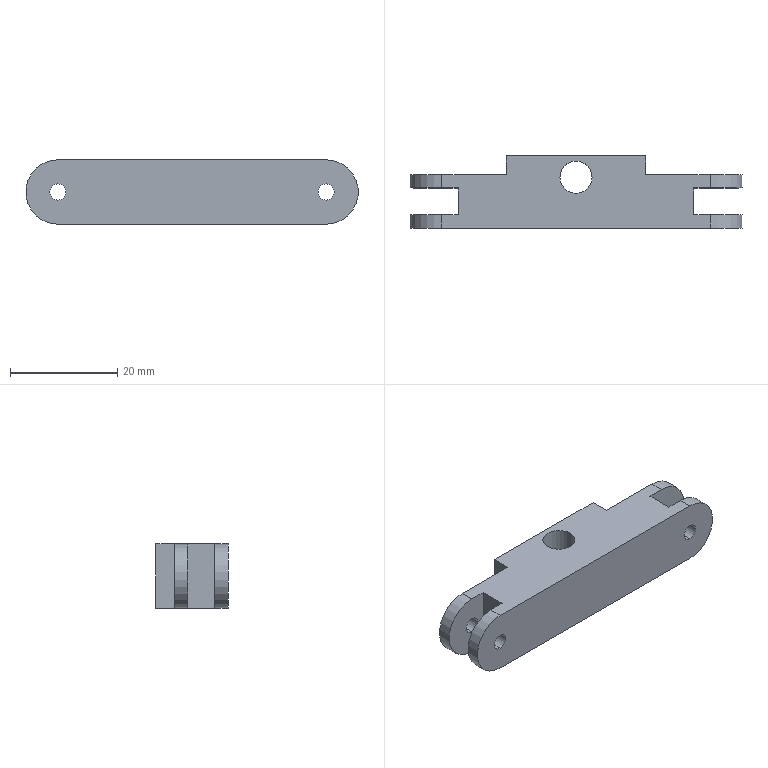Part | SolidWorks | features ICE 4, Extrusion 1, MirrorSolid 1 | 1 solid | 28 faces | box 62 x 13.5 x 12 mm | volume 6888 mm3 | cylinder 14 | plane 14 | commonest cylinder face diameters 3 x8 12 x4 6 x2
STEP:
#1=CARTESIAN_POINT('',(22.,9.5,-6.));
#2=VERTEX_POINT('',#1);
#3=CARTESIAN_POINT('',(28.,9.5,-6.));
#4=VERTEX_POINT('',#3);
#5=CARTESIAN_POINT('',(25.,9.5,-6.));
#6=DIRECTION('',(0.,0.,1.));
#7=DIRECTION('',(1.,0.,0.));
#8=AXIS2_PLACEMENT_3D('',#5,#6,#7);
#9=CIRCLE('',#8,3.);
#10=EDGE_CURVE('',#2,#4,#9,.T.);
#11=ORIENTED_EDGE('',*,*,#10,.F.);
#12=CARTESIAN_POINT('',(22.,9.5,6.));
#13=VERTEX_POINT('',#12);
#14=CARTESIAN_POINT('',(22.,9.5,-6.));
#15=DIRECTION('',(0.,0.,1.));
#16=VECTOR('',#15,1000.);
#17=LINE('',#14,#16);
#18=EDGE_CURVE('',#2,#13,#17,.T.);
#19=ORIENTED_EDGE('',*,*,#18,.T.);
#20=CARTESIAN_POINT('',(28.,9.5,6.));
#21=VERTEX_POINT('',#20);
#22=CARTESIAN_POINT('',(25.,9.5,6.));
#23=DIRECTION('',(0.,0.,1.));
#24=DIRECTION('',(1.,0.,0.));
#25=AXIS2_PLACEMENT_3D('',#22,#23,#24);
#26=CIRCLE('',#25,3.);
#27=EDGE_CURVE('',#13,#21,#26,.T.);
#28=ORIENTED_EDGE('',*,*,#27,.T.);
#29=CARTESIAN_POINT('',(28.,9.5,-6.));
#30=DIRECTION('',(0.,0.,1.));
#31=VECTOR('',#30,1000.);
#32=LINE('',#29,#31);
#33=EDGE_CURVE('',#4,#21,#32,.T.);
#34=ORIENTED_EDGE('',*,*,#33,.F.);
#35=EDGE_LOOP('',(#11,#19,#28,#34));
#36=FACE_OUTER_BOUND('',#35,.T.);
#37=CARTESIAN_POINT('',(25.,9.5,-6.));
#38=DIRECTION('',(0.,0.,1.));
#39=DIRECTION('',(1.,0.,0.));
#40=AXIS2_PLACEMENT_3D('',#37,#38,#39);
#41=CYLINDRICAL_SURFACE('',#40,3.);
#42=ADVANCED_FACE('',(#36),#41,.F.);
#43=CARTESIAN_POINT('',(50.,2.5,-1.5));
#44=VERTEX_POINT('',#43);
#45=CARTESIAN_POINT('',(50.,2.5,1.5));
#46=VERTEX_POINT('',#45);
#47=CARTESIAN_POINT('',(50.,2.5,0.));
#48=DIRECTION('',(0.,1.,0.));
#49=DIRECTION('',(-1.,0.,0.));
#50=AXIS2_PLACEMENT_3D('',#47,#48,#49);
#51=CIRCLE('',#50,1.5);
#52=EDGE_CURVE('',#44,#46,#51,.T.);
#53=ORIENTED_EDGE('',*,*,#52,.T.);
#54=CARTESIAN_POINT('',(50.,0.,1.5));
#55=VERTEX_POINT('',#54);
#56=CARTESIAN_POINT('',(50.,10.,1.5));
#57=DIRECTION('',(0.,-1.,0.));
#58=VECTOR('',#57,1000.);
#59=LINE('',#56,#58);
#60=EDGE_CURVE('',#46,#55,#59,.T.);
#61=ORIENTED_EDGE('',*,*,#60,.T.);
#62=CARTESIAN_POINT('',(50.,0.,-1.5));
#63=VERTEX_POINT('',#62);
#64=CARTESIAN_POINT('',(50.,0.,0.));
#65=DIRECTION('',(0.,-1.,0.));
#66=DIRECTION('',(0.,0.,1.));
#67=AXIS2_PLACEMENT_3D('',#64,#65,#66);
#68=CIRCLE('',#67,1.5);
#69=EDGE_CURVE('',#55,#63,#68,.T.);
#70=ORIENTED_EDGE('',*,*,#69,.T.);
#71=CARTESIAN_POINT('',(50.,10.,-1.5));
#72=DIRECTION('',(0.,-1.,0.));
#73=VECTOR('',#72,1000.);
#74=LINE('',#71,#73);
#75=EDGE_CURVE('',#44,#63,#74,.T.);
#76=ORIENTED_EDGE('',*,*,#75,.F.);
#77=EDGE_LOOP('',(#53,#61,#70,#76));
#78=FACE_OUTER_BOUND('',#77,.T.);
#79=CARTESIAN_POINT('',(50.,10.,0.));
#80=DIRECTION('',(0.,-1.,0.));
#81=DIRECTION('',(0.,0.,-1.));
#82=AXIS2_PLACEMENT_3D('',#79,#80,#81);
#83=CYLINDRICAL_SURFACE('',#82,1.5);
#84=ADVANCED_FACE('',(#78),#83,.F.);
#85=CARTESIAN_POINT('',(50.,10.,1.5));
#86=VERTEX_POINT('',#85);
#87=CARTESIAN_POINT('',(50.,10.,-1.5));
#88=VERTEX_POINT('',#87);
#89=CARTESIAN_POINT('',(50.,10.,0.));
#90=DIRECTION('',(0.,-1.,0.));
#91=DIRECTION('',(0.,0.,1.));
#92=AXIS2_PLACEMENT_3D('',#89,#90,#91);
#93=CIRCLE('',#92,1.5);
#94=EDGE_CURVE('',#86,#88,#93,.T.);
#95=ORIENTED_EDGE('',*,*,#94,.F.);
#96=CARTESIAN_POINT('',(50.,7.5,1.5));
#97=VERTEX_POINT('',#96);
#98=CARTESIAN_POINT('',(50.,10.,1.5));
#99=DIRECTION('',(0.,-1.,0.));
#100=VECTOR('',#99,1000.);
#101=LINE('',#98,#100);
#102=EDGE_CURVE('',#86,#97,#101,.T.);
#103=ORIENTED_EDGE('',*,*,#102,.T.);
#104=CARTESIAN_POINT('',(50.,7.5,-1.5));
#105=VERTEX_POINT('',#104);
#106=CARTESIAN_POINT('',(50.,7.5,0.));
#107=DIRECTION('',(0.,-1.,0.));
#108=DIRECTION('',(1.,0.,0.));
#109=AXIS2_PLACEMENT_3D('',#106,#107,#108);
#110=CIRCLE('',#109,1.5);
#111=EDGE_CURVE('',#97,#105,#110,.T.);
#112=ORIENTED_EDGE('',*,*,#111,.T.);
#113=CARTESIAN_POINT('',(50.,10.,-1.5));
#114=DIRECTION('',(0.,-1.,0.));
#115=VECTOR('',#114,1000.);
#116=LINE('',#113,#115);
#117=EDGE_CURVE('',#88,#105,#116,.T.);
#118=ORIENTED_EDGE('',*,*,#117,.F.);
#119=EDGE_LOOP('',(#95,#103,#112,#118));
#120=FACE_OUTER_BOUND('',#119,.T.);
#121=CARTESIAN_POINT('',(50.,10.,0.));
#122=DIRECTION('',(0.,-1.,0.));
#123=DIRECTION('',(0.,0.,-1.));
#124=AXIS2_PLACEMENT_3D('',#121,#122,#123);
#125=CYLINDRICAL_SURFACE('',#124,1.5);
#126=ADVANCED_FACE('',(#120),#125,.F.);
#127=CARTESIAN_POINT('',(0.,2.5,1.5));
#128=VERTEX_POINT('',#127);
#129=CARTESIAN_POINT('',(0.,2.5,-1.5));
#130=VERTEX_POINT('',#129);
#131=CARTESIAN_POINT('',(0.,2.5,0.));
#132=DIRECTION('',(0.,-1.,0.));
#133=DIRECTION('',(1.,0.,0.));
#134=AXIS2_PLACEMENT_3D('',#131,#132,#133);
#135=CIRCLE('',#134,1.5);
#136=EDGE_CURVE('',#128,#130,#135,.T.);
#137=ORIENTED_EDGE('',*,*,#136,.F.);
#138=CARTESIAN_POINT('',(0.,0.,1.5));
#139=VERTEX_POINT('',#138);
#140=CARTESIAN_POINT('',(0.,10.,1.5));
#141=DIRECTION('',(0.,-1.,0.));
#142=VECTOR('',#141,1000.);
#143=LINE('',#140,#142);
#144=EDGE_CURVE('',#128,#139,#143,.T.);
#145=ORIENTED_EDGE('',*,*,#144,.T.);
#146=CARTESIAN_POINT('',(0.,0.,-1.5));
#147=VERTEX_POINT('',#146);
#148=CARTESIAN_POINT('',(0.,0.,0.));
#149=DIRECTION('',(0.,1.,0.));
#150=DIRECTION('',(0.,0.,1.));
#151=AXIS2_PLACEMENT_3D('',#148,#149,#150);
#152=CIRCLE('',#151,1.5);
#153=EDGE_CURVE('',#147,#139,#152,.T.);
#154=ORIENTED_EDGE('',*,*,#153,.F.);
#155=CARTESIAN_POINT('',(0.,10.,-1.5));
#156=DIRECTION('',(0.,-1.,0.));
#157=VECTOR('',#156,1000.);
#158=LINE('',#155,#157);
#159=EDGE_CURVE('',#130,#147,#158,.T.);
#160=ORIENTED_EDGE('',*,*,#159,.F.);
#161=EDGE_LOOP('',(#137,#145,#154,#160));
#162=FACE_OUTER_BOUND('',#161,.T.);
#163=CARTESIAN_POINT('',(0.,10.,0.));
#164=DIRECTION('',(0.,-1.,0.));
#165=DIRECTION('',(0.,0.,-1.));
#166=AXIS2_PLACEMENT_3D('',#163,#164,#165);
#167=CYLINDRICAL_SURFACE('',#166,1.5);
#168=ADVANCED_FACE('',(#162),#167,.F.);
#169=CARTESIAN_POINT('',(0.,10.,-1.5));
#170=VERTEX_POINT('',#169);
#171=CARTESIAN_POINT('',(0.,10.,1.5));
#172=VERTEX_POINT('',#171);
#173=CARTESIAN_POINT('',(0.,10.,0.));
#174=DIRECTION('',(0.,1.,0.));
#175=DIRECTION('',(0.,0.,1.));
#176=AXIS2_PLACEMENT_3D('',#173,#174,#175);
#177=CIRCLE('',#176,1.5);
#178=EDGE_CURVE('',#170,#172,#177,.T.);
#179=ORIENTED_EDGE('',*,*,#178,.T.);
#180=CARTESIAN_POINT('',(0.,7.5,1.5));
#181=VERTEX_POINT('',#180);
#182=CARTESIAN_POINT('',(0.,10.,1.5));
#183=DIRECTION('',(0.,-1.,0.));
#184=VECTOR('',#183,1000.);
#185=LINE('',#182,#184);
#186=EDGE_CURVE('',#172,#181,#185,.T.);
#187=ORIENTED_EDGE('',*,*,#186,.T.);
#188=CARTESIAN_POINT('',(0.,7.5,-1.5));
#189=VERTEX_POINT('',#188);
#190=CARTESIAN_POINT('',(0.,7.5,0.));
#191=DIRECTION('',(0.,1.,0.));
#192=DIRECTION('',(-1.,0.,0.));
#193=AXIS2_PLACEMENT_3D('',#190,#191,#192);
#194=CIRCLE('',#193,1.5);
#195=EDGE_CURVE('',#189,#181,#194,.T.);
#196=ORIENTED_EDGE('',*,*,#195,.F.);
#197=CARTESIAN_POINT('',(0.,10.,-1.5));
#198=DIRECTION('',(0.,-1.,0.));
#199=VECTOR('',#198,1000.);
#200=LINE('',#197,#199);
#201=EDGE_CURVE('',#170,#189,#200,.T.);
#202=ORIENTED_EDGE('',*,*,#201,.F.);
#203=EDGE_LOOP('',(#179,#187,#196,#202));
#204=FACE_OUTER_BOUND('',#203,.T.);
#205=CARTESIAN_POINT('',(0.,10.,0.));
#206=DIRECTION('',(0.,-1.,0.));
#207=DIRECTION('',(0.,0.,-1.));
#208=AXIS2_PLACEMENT_3D('',#205,#206,#207);
#209=CYLINDRICAL_SURFACE('',#208,1.5);
#210=ADVANCED_FACE('',(#204),#209,.F.);
#211=CARTESIAN_POINT('',(0.,7.5,-6.));
#212=VERTEX_POINT('',#211);
#213=CARTESIAN_POINT('',(0.,7.5,6.));
#214=VERTEX_POINT('',#213);
#215=CARTESIAN_POINT('',(0.,7.5,0.));
#216=DIRECTION('',(0.,1.,0.));
#217=DIRECTION('',(-1.,0.,0.));
#218=AXIS2_PLACEMENT_3D('',#215,#216,#217);
#219=CIRCLE('',#218,6.);
#220=EDGE_CURVE('',#212,#214,#219,.T.);
#221=ORIENTED_EDGE('',*,*,#220,.T.);
#222=CARTESIAN_POINT('',(0.,10.,6.));
#223=VERTEX_POINT('',#222);
#224=CARTESIAN_POINT('',(0.,10.,6.));
#225=DIRECTION('',(0.,-1.,0.));
#226=VECTOR('',#225,1000.);
#227=LINE('',#224,#226);
#228=EDGE_CURVE('',#223,#214,#227,.T.);
#229=ORIENTED_EDGE('',*,*,#228,.F.);
#230=CARTESIAN_POINT('',(0.,10.,-6.));
#231=VERTEX_POINT('',#230);
#232=CARTESIAN_POINT('',(0.,10.,0.));
#233=DIRECTION('',(0.,1.,0.));
#234=DIRECTION('',(0.,0.,1.));
#235=AXIS2_PLACEMENT_3D('',#232,#233,#234);
#236=CIRCLE('',#235,6.);
#237=EDGE_CURVE('',#231,#223,#236,.T.);
#238=ORIENTED_EDGE('',*,*,#237,.F.);
#239=CARTESIAN_POINT('',(0.,10.,-6.));
#240=DIRECTION('',(0.,-1.,0.));
#241=VECTOR('',#240,1000.);
#242=LINE('',#239,#241);
#243=EDGE_CURVE('',#231,#212,#242,.T.);
#244=ORIENTED_EDGE('',*,*,#243,.T.);
#245=EDGE_LOOP('',(#221,#229,#238,#244));
#246=FACE_OUTER_BOUND('',#245,.T.);
#247=CARTESIAN_POINT('',(0.,10.,0.));
#248=DIRECTION('',(0.,-1.,0.));
#249=DIRECTION('',(0.,0.,-1.));
#250=AXIS2_PLACEMENT_3D('',#247,#248,#249);
#251=CYLINDRICAL_SURFACE('',#250,6.);
#252=ADVANCED_FACE('',(#246),#251,.T.);
#253=ORIENTED_EDGE('',*,*,#186,.F.);
#254=CARTESIAN_POINT('',(0.,10.,0.));
#255=DIRECTION('',(0.,1.,0.));
#256=DIRECTION('',(0.,0.,1.));
#257=AXIS2_PLACEMENT_3D('',#254,#255,#256);
#258=CIRCLE('',#257,1.5);
#259=EDGE_CURVE('',#172,#170,#258,.T.);
#260=ORIENTED_EDGE('',*,*,#259,.T.);
#261=ORIENTED_EDGE('',*,*,#201,.T.);
#262=CARTESIAN_POINT('',(0.,7.5,0.));
#263=DIRECTION('',(0.,1.,0.));
#264=DIRECTION('',(-1.,0.,0.));
#265=AXIS2_PLACEMENT_3D('',#262,#263,#264);
#266=CIRCLE('',#265,1.5);
#267=EDGE_CURVE('',#181,#189,#266,.T.);
#268=ORIENTED_EDGE('',*,*,#267,.F.);
#269=EDGE_LOOP('',(#253,#260,#261,#268));
#270=FACE_OUTER_BOUND('',#269,.T.);
#271=CARTESIAN_POINT('',(0.,10.,0.));
#272=DIRECTION('',(0.,-1.,0.));
#273=DIRECTION('',(0.,0.,-1.));
#274=AXIS2_PLACEMENT_3D('',#271,#272,#273);
#275=CYLINDRICAL_SURFACE('',#274,1.5);
#276=ADVANCED_FACE('',(#270),#275,.F.);
#277=CARTESIAN_POINT('',(12.,10.,-6.));
#278=VERTEX_POINT('',#277);
#279=CARTESIAN_POINT('',(12.,10.,6.));
#280=VERTEX_POINT('',#279);
#281=CARTESIAN_POINT('',(12.,10.,0.));
#282=DIRECTION('',(0.,0.,1.));
#283=VECTOR('',#282,1000.);
#284=LINE('',#281,#283);
#285=EDGE_CURVE('',#278,#280,#284,.T.);
#286=ORIENTED_EDGE('',*,*,#285,.F.);
#287=CARTESIAN_POINT('',(0.,10.,-6.));
#288=DIRECTION('',(-1.,0.,0.));
#289=VECTOR('',#288,1000.);
#290=LINE('',#287,#289);
#291=EDGE_CURVE('',#278,#231,#290,.T.);
#292=ORIENTED_EDGE('',*,*,#291,.T.);
#293=ORIENTED_EDGE('',*,*,#237,.T.);
#294=CARTESIAN_POINT('',(0.,10.,6.));
#295=DIRECTION('',(1.,0.,0.));
#296=VECTOR('',#295,1000.);
#297=LINE('',#294,#296);
#298=EDGE_CURVE('',#223,#280,#297,.T.);
#299=ORIENTED_EDGE('',*,*,#298,.T.);
#300=EDGE_LOOP('',(#286,#292,#293,#299));
#301=FACE_OUTER_BOUND('',#300,.T.);
#302=ORIENTED_EDGE('',*,*,#178,.F.);
#303=ORIENTED_EDGE('',*,*,#259,.F.);
#304=EDGE_LOOP('',(#302,#303));
#305=FACE_BOUND('',#304,.T.);
#306=CARTESIAN_POINT('',(0.,10.,0.));
#307=DIRECTION('',(0.,1.,0.));
#308=DIRECTION('',(0.,0.,1.));
#309=AXIS2_PLACEMENT_3D('',#306,#307,#308);
#310=PLANE('',#309);
#311=ADVANCED_FACE('',(#301,#305),#310,.T.);
#312=CARTESIAN_POINT('',(50.,0.,-6.));
#313=VERTEX_POINT('',#312);
#314=CARTESIAN_POINT('',(0.,0.,-6.));
#315=VERTEX_POINT('',#314);
#316=CARTESIAN_POINT('',(0.,0.,-6.));
#317=DIRECTION('',(-1.,0.,0.));
#318=VECTOR('',#317,1000.);
#319=LINE('',#316,#318);
#320=EDGE_CURVE('',#313,#315,#319,.T.);
#321=ORIENTED_EDGE('',*,*,#320,.F.);
#322=CARTESIAN_POINT('',(50.,0.,6.));
#323=VERTEX_POINT('',#322);
#324=CARTESIAN_POINT('',(50.,0.,0.));
#325=DIRECTION('',(0.,-1.,0.));
#326=DIRECTION('',(0.,0.,1.));
#327=AXIS2_PLACEMENT_3D('',#324,#325,#326);
#328=CIRCLE('',#327,6.);
#329=EDGE_CURVE('',#313,#323,#328,.T.);
#330=ORIENTED_EDGE('',*,*,#329,.T.);
#331=CARTESIAN_POINT('',(0.,0.,6.));
#332=VERTEX_POINT('',#331);
#333=CARTESIAN_POINT('',(0.,0.,6.));
#334=DIRECTION('',(1.,0.,0.));
#335=VECTOR('',#334,1000.);
#336=LINE('',#333,#335);
#337=EDGE_CURVE('',#332,#323,#336,.T.);
#338=ORIENTED_EDGE('',*,*,#337,.F.);
#339=CARTESIAN_POINT('',(0.,0.,0.));
#340=DIRECTION('',(0.,1.,0.));
#341=DIRECTION('',(0.,0.,1.));
#342=AXIS2_PLACEMENT_3D('',#339,#340,#341);
#343=CIRCLE('',#342,6.);
#344=EDGE_CURVE('',#315,#332,#343,.T.);
#345=ORIENTED_EDGE('',*,*,#344,.F.);
#346=EDGE_LOOP('',(#321,#330,#338,#345));
#347=FACE_OUTER_BOUND('',#346,.T.);
#348=ORIENTED_EDGE('',*,*,#153,.T.);
#349=CARTESIAN_POINT('',(0.,0.,0.));
#350=DIRECTION('',(0.,1.,0.));
#351=DIRECTION('',(0.,0.,1.));
#352=AXIS2_PLACEMENT_3D('',#349,#350,#351);
#353=CIRCLE('',#352,1.5);
#354=EDGE_CURVE('',#139,#147,#353,.T.);
#355=ORIENTED_EDGE('',*,*,#354,.T.);
#356=EDGE_LOOP('',(#348,#355));
#357=FACE_BOUND('',#356,.T.);
#358=CARTESIAN_POINT('',(50.,0.,0.));
#359=DIRECTION('',(0.,-1.,0.));
#360=DIRECTION('',(0.,0.,1.));
#361=AXIS2_PLACEMENT_3D('',#358,#359,#360);
#362=CIRCLE('',#361,1.5);
#363=EDGE_CURVE('',#63,#55,#362,.T.);
#364=ORIENTED_EDGE('',*,*,#363,.F.);
#365=ORIENTED_EDGE('',*,*,#69,.F.);
#366=EDGE_LOOP('',(#364,#365));
#367=FACE_BOUND('',#366,.T.);
#368=CARTESIAN_POINT('',(0.,0.,0.));
#369=DIRECTION('',(0.,1.,0.));
#370=DIRECTION('',(0.,0.,1.));
#371=AXIS2_PLACEMENT_3D('',#368,#369,#370);
#372=PLANE('',#371);
#373=ADVANCED_FACE('',(#347,#357,#367),#372,.F.);
#374=CARTESIAN_POINT('',(0.,2.5,6.));
#375=VERTEX_POINT('',#374);
#376=CARTESIAN_POINT('',(0.,10.,6.));
#377=DIRECTION('',(0.,-1.,0.));
#378=VECTOR('',#377,1000.);
#379=LINE('',#376,#378);
#380=EDGE_CURVE('',#375,#332,#379,.T.);
#381=ORIENTED_EDGE('',*,*,#380,.F.);
#382=CARTESIAN_POINT('',(0.,2.5,-6.));
#383=VERTEX_POINT('',#382);
#384=CARTESIAN_POINT('',(0.,2.5,0.));
#385=DIRECTION('',(0.,-1.,0.));
#386=DIRECTION('',(1.,0.,0.));
#387=AXIS2_PLACEMENT_3D('',#384,#385,#386);
#388=CIRCLE('',#387,6.);
#389=EDGE_CURVE('',#375,#383,#388,.T.);
#390=ORIENTED_EDGE('',*,*,#389,.T.);
#391=CARTESIAN_POINT('',(0.,10.,-6.));
#392=DIRECTION('',(0.,-1.,0.));
#393=VECTOR('',#392,1000.);
#394=LINE('',#391,#393);
#395=EDGE_CURVE('',#383,#315,#394,.T.);
#396=ORIENTED_EDGE('',*,*,#395,.T.);
#397=ORIENTED_EDGE('',*,*,#344,.T.);
#398=EDGE_LOOP('',(#381,#390,#396,#397));
#399=FACE_OUTER_BOUND('',#398,.T.);
#400=CARTESIAN_POINT('',(0.,10.,0.));
#401=DIRECTION('',(0.,-1.,0.));
#402=DIRECTION('',(0.,0.,-1.));
#403=AXIS2_PLACEMENT_3D('',#400,#401,#402);
#404=CYLINDRICAL_SURFACE('',#403,6.);
#405=ADVANCED_FACE('',(#399),#404,.T.);
#406=CARTESIAN_POINT('',(25.,9.5,6.));
#407=DIRECTION('',(0.,0.,1.));
#408=DIRECTION('',(1.,0.,0.));
#409=AXIS2_PLACEMENT_3D('',#406,#407,#408);
#410=CIRCLE('',#409,3.);
#411=EDGE_CURVE('',#21,#13,#410,.T.);
#412=ORIENTED_EDGE('',*,*,#411,.F.);
#413=ORIENTED_EDGE('',*,*,#27,.F.);
#414=EDGE_LOOP('',(#412,#413));
#415=FACE_BOUND('',#414,.T.);
#416=CARTESIAN_POINT('',(12.,13.5,6.));
#417=VERTEX_POINT('',#416);
#418=CARTESIAN_POINT('',(12.,7.5,6.));
#419=DIRECTION('',(0.,-1.,0.));
#420=VECTOR('',#419,1000.);
#421=LINE('',#418,#420);
#422=EDGE_CURVE('',#417,#280,#421,.T.);
#423=ORIENTED_EDGE('',*,*,#422,.T.);
#424=ORIENTED_EDGE('',*,*,#298,.F.);
#425=ORIENTED_EDGE('',*,*,#228,.T.);
#426=CARTESIAN_POINT('',(3.,7.5,6.));
#427=VERTEX_POINT('',#426);
#428=CARTESIAN_POINT('',(-6.,7.5,6.));
#429=DIRECTION('',(-1.,0.,0.));
#430=VECTOR('',#429,1000.);
#431=LINE('',#428,#430);
#432=EDGE_CURVE('',#427,#214,#431,.T.);
#433=ORIENTED_EDGE('',*,*,#432,.F.);
#434=CARTESIAN_POINT('',(3.,2.5,6.));
#435=VERTEX_POINT('',#434);
#436=CARTESIAN_POINT('',(3.,7.5,6.));
#437=DIRECTION('',(0.,1.,0.));
#438=VECTOR('',#437,1000.);
#439=LINE('',#436,#438);
#440=EDGE_CURVE('',#435,#427,#439,.T.);
#441=ORIENTED_EDGE('',*,*,#440,.F.);
#442=CARTESIAN_POINT('',(-6.,2.5,6.));
#443=DIRECTION('',(1.,0.,0.));
#444=VECTOR('',#443,1000.);
#445=LINE('',#442,#444);
#446=EDGE_CURVE('',#375,#435,#445,.T.);
#447=ORIENTED_EDGE('',*,*,#446,.F.);
#448=ORIENTED_EDGE('',*,*,#380,.T.);
#449=ORIENTED_EDGE('',*,*,#337,.T.);
#450=CARTESIAN_POINT('',(50.,2.5,6.));
#451=VERTEX_POINT('',#450);
#452=CARTESIAN_POINT('',(50.,10.,6.));
#453=DIRECTION('',(0.,-1.,0.));
#454=VECTOR('',#453,1000.);
#455=LINE('',#452,#454);
#456=EDGE_CURVE('',#451,#323,#455,.T.);
#457=ORIENTED_EDGE('',*,*,#456,.F.);
#458=CARTESIAN_POINT('',(47.,2.5,6.));
#459=VERTEX_POINT('',#458);
#460=CARTESIAN_POINT('',(56.,2.5,6.));
#461=DIRECTION('',(-1.,0.,0.));
#462=VECTOR('',#461,1000.);
#463=LINE('',#460,#462);
#464=EDGE_CURVE('',#451,#459,#463,.T.);
#465=ORIENTED_EDGE('',*,*,#464,.T.);
#466=CARTESIAN_POINT('',(47.,7.5,6.));
#467=VERTEX_POINT('',#466);
#468=CARTESIAN_POINT('',(47.,7.5,6.));
#469=DIRECTION('',(0.,1.,0.));
#470=VECTOR('',#469,1000.);
#471=LINE('',#468,#470);
#472=EDGE_CURVE('',#459,#467,#471,.T.);
#473=ORIENTED_EDGE('',*,*,#472,.T.);
#474=CARTESIAN_POINT('',(50.,7.5,6.));
#475=VERTEX_POINT('',#474);
#476=CARTESIAN_POINT('',(56.,7.5,6.));
#477=DIRECTION('',(1.,0.,0.));
#478=VECTOR('',#477,1000.);
#479=LINE('',#476,#478);
#480=EDGE_CURVE('',#467,#475,#479,.T.);
#481=ORIENTED_EDGE('',*,*,#480,.T.);
#482=CARTESIAN_POINT('',(50.,10.,6.));
#483=VERTEX_POINT('',#482);
#484=CARTESIAN_POINT('',(50.,10.,6.));
#485=DIRECTION('',(0.,-1.,0.));
#486=VECTOR('',#485,1000.);
#487=LINE('',#484,#486);
#488=EDGE_CURVE('',#483,#475,#487,.T.);
#489=ORIENTED_EDGE('',*,*,#488,.F.);
#490=CARTESIAN_POINT('',(38.,10.,6.));
#491=VERTEX_POINT('',#490);
#492=CARTESIAN_POINT('',(50.,10.,6.));
#493=DIRECTION('',(-1.,0.,0.));
#494=VECTOR('',#493,1000.);
#495=LINE('',#492,#494);
#496=EDGE_CURVE('',#483,#491,#495,.T.);
#497=ORIENTED_EDGE('',*,*,#496,.T.);
#498=CARTESIAN_POINT('',(38.,13.5,6.));
#499=VERTEX_POINT('',#498);
#500=CARTESIAN_POINT('',(38.,7.5,6.));
#501=DIRECTION('',(0.,1.,0.));
#502=VECTOR('',#501,1000.);
#503=LINE('',#500,#502);
#504=EDGE_CURVE('',#491,#499,#503,.T.);
#505=ORIENTED_EDGE('',*,*,#504,.T.);
#506=CARTESIAN_POINT('',(12.,13.5,6.));
#507=DIRECTION('',(-1.,0.,0.));
#508=VECTOR('',#507,1000.);
#509=LINE('',#506,#508);
#510=EDGE_CURVE('',#499,#417,#509,.T.);
#511=ORIENTED_EDGE('',*,*,#510,.T.);
#512=EDGE_LOOP('',(#423,#424,#425,#433,#441,#447,#448,#449,#457,#465,#473,#481,#489,#497,#505,#511));
#513=FACE_OUTER_BOUND('',#512,.T.);
#514=CARTESIAN_POINT('',(0.,10.,6.));
#515=DIRECTION('',(0.,0.,-1.));
#516=DIRECTION('',(-1.,0.,0.));
#517=AXIS2_PLACEMENT_3D('',#514,#515,#516);
#518=PLANE('',#517);
#519=ADVANCED_FACE('',(#415,#513),#518,.F.);
#520=CARTESIAN_POINT('',(25.,9.5,-6.));
#521=DIRECTION('',(0.,0.,1.));
#522=DIRECTION('',(1.,0.,0.));
#523=AXIS2_PLACEMENT_3D('',#520,#521,#522);
#524=CIRCLE('',#523,3.);
#525=EDGE_CURVE('',#4,#2,#524,.T.);
#526=ORIENTED_EDGE('',*,*,#525,.T.);
#527=ORIENTED_EDGE('',*,*,#10,.T.);
#528=EDGE_LOOP('',(#526,#527));
#529=FACE_BOUND('',#528,.T.);
#530=ORIENTED_EDGE('',*,*,#291,.F.);
#531=CARTESIAN_POINT('',(12.,13.5,-6.));
#532=VERTEX_POINT('',#531);
#533=CARTESIAN_POINT('',(12.,7.5,-6.));
#534=DIRECTION('',(0.,1.,0.));
#535=VECTOR('',#534,1000.);
#536=LINE('',#533,#535);
#537=EDGE_CURVE('',#278,#532,#536,.T.);
#538=ORIENTED_EDGE('',*,*,#537,.T.);
#539=CARTESIAN_POINT('',(38.,13.5,-6.));
#540=VERTEX_POINT('',#539);
#541=CARTESIAN_POINT('',(12.,13.5,-6.));
#542=DIRECTION('',(1.,0.,0.));
#543=VECTOR('',#542,1000.);
#544=LINE('',#541,#543);
#545=EDGE_CURVE('',#532,#540,#544,.T.);
#546=ORIENTED_EDGE('',*,*,#545,.T.);
#547=CARTESIAN_POINT('',(38.,10.,-6.));
#548=VERTEX_POINT('',#547);
#549=CARTESIAN_POINT('',(38.,7.5,-6.));
#550=DIRECTION('',(0.,-1.,0.));
#551=VECTOR('',#550,1000.);
#552=LINE('',#549,#551);
#553=EDGE_CURVE('',#540,#548,#552,.T.);
#554=ORIENTED_EDGE('',*,*,#553,.T.);
#555=CARTESIAN_POINT('',(50.,10.,-6.));
#556=VERTEX_POINT('',#555);
#557=CARTESIAN_POINT('',(50.,10.,-6.));
#558=DIRECTION('',(1.,0.,0.));
#559=VECTOR('',#558,1000.);
#560=LINE('',#557,#559);
#561=EDGE_CURVE('',#548,#556,#560,.T.);
#562=ORIENTED_EDGE('',*,*,#561,.T.);
#563=CARTESIAN_POINT('',(50.,7.5,-6.));
#564=VERTEX_POINT('',#563);
#565=CARTESIAN_POINT('',(50.,10.,-6.));
#566=DIRECTION('',(0.,-1.,0.));
#567=VECTOR('',#566,1000.);
#568=LINE('',#565,#567);
#569=EDGE_CURVE('',#556,#564,#568,.T.);
#570=ORIENTED_EDGE('',*,*,#569,.T.);
#571=CARTESIAN_POINT('',(47.,7.5,-6.));
#572=VERTEX_POINT('',#571);
#573=CARTESIAN_POINT('',(56.,7.5,-6.));
#574=DIRECTION('',(1.,0.,0.));
#575=VECTOR('',#574,1000.);
#576=LINE('',#573,#575);
#577=EDGE_CURVE('',#572,#564,#576,.T.);
#578=ORIENTED_EDGE('',*,*,#577,.F.);
#579=CARTESIAN_POINT('',(47.,2.5,-6.));
#580=VERTEX_POINT('',#579);
#581=CARTESIAN_POINT('',(47.,7.5,-6.));
#582=DIRECTION('',(0.,1.,0.));
#583=VECTOR('',#582,1000.);
#584=LINE('',#581,#583);
#585=EDGE_CURVE('',#580,#572,#584,.T.);
#586=ORIENTED_EDGE('',*,*,#585,.F.);
#587=CARTESIAN_POINT('',(50.,2.5,-6.));
#588=VERTEX_POINT('',#587);
#589=CARTESIAN_POINT('',(56.,2.5,-6.));
#590=DIRECTION('',(-1.,0.,0.));
#591=VECTOR('',#590,1000.);
#592=LINE('',#589,#591);
#593=EDGE_CURVE('',#588,#580,#592,.T.);
#594=ORIENTED_EDGE('',*,*,#593,.F.);
#595=CARTESIAN_POINT('',(50.,10.,-6.));
#596=DIRECTION('',(0.,-1.,0.));
#597=VECTOR('',#596,1000.);
#598=LINE('',#595,#597);
#599=EDGE_CURVE('',#588,#313,#598,.T.);
#600=ORIENTED_EDGE('',*,*,#599,.T.);
#601=ORIENTED_EDGE('',*,*,#320,.T.);
#602=ORIENTED_EDGE('',*,*,#395,.F.);
#603=CARTESIAN_POINT('',(3.,2.5,-6.));
#604=VERTEX_POINT('',#603);
#605=CARTESIAN_POINT('',(-6.,2.5,-6.));
#606=DIRECTION('',(1.,0.,0.));
#607=VECTOR('',#606,1000.);
#608=LINE('',#605,#607);
#609=EDGE_CURVE('',#383,#604,#608,.T.);
#610=ORIENTED_EDGE('',*,*,#609,.T.);
#611=CARTESIAN_POINT('',(3.,7.5,-6.));
#612=VERTEX_POINT('',#611);
#613=CARTESIAN_POINT('',(3.,7.5,-6.));
#614=DIRECTION('',(0.,1.,0.));
#615=VECTOR('',#614,1000.);
#616=LINE('',#613,#615);
#617=EDGE_CURVE('',#604,#612,#616,.T.);
#618=ORIENTED_EDGE('',*,*,#617,.T.);
#619=CARTESIAN_POINT('',(-6.,7.5,-6.));
#620=DIRECTION('',(-1.,0.,0.));
#621=VECTOR('',#620,1000.);
#622=LINE('',#619,#621);
#623=EDGE_CURVE('',#612,#212,#622,.T.);
#624=ORIENTED_EDGE('',*,*,#623,.T.);
#625=ORIENTED_EDGE('',*,*,#243,.F.);
#626=EDGE_LOOP('',(#530,#538,#546,#554,#562,#570,#578,#586,#594,#600,#601,#602,#610,#618,#624,#625));
#627=FACE_OUTER_BOUND('',#626,.T.);
#628=CARTESIAN_POINT('',(0.,10.,-6.));
#629=DIRECTION('',(0.,0.,1.));
#630=DIRECTION('',(1.,0.,0.));
#631=AXIS2_PLACEMENT_3D('',#628,#629,#630);
#632=PLANE('',#631);
#633=ADVANCED_FACE('',(#529,#627),#632,.F.);
#634=ORIENTED_EDGE('',*,*,#144,.F.);
#635=CARTESIAN_POINT('',(0.,2.5,0.));
#636=DIRECTION('',(0.,-1.,0.));
#637=DIRECTION('',(1.,0.,0.));
#638=AXIS2_PLACEMENT_3D('',#635,#636,#637);
#639=CIRCLE('',#638,1.5);
#640=EDGE_CURVE('',#130,#128,#639,.T.);
#641=ORIENTED_EDGE('',*,*,#640,.F.);
#642=ORIENTED_EDGE('',*,*,#159,.T.);
#643=ORIENTED_EDGE('',*,*,#354,.F.);
#644=EDGE_LOOP('',(#634,#641,#642,#643));
#645=FACE_OUTER_BOUND('',#644,.T.);
#646=CARTESIAN_POINT('',(0.,10.,0.));
#647=DIRECTION('',(0.,-1.,0.));
#648=DIRECTION('',(0.,0.,-1.));
#649=AXIS2_PLACEMENT_3D('',#646,#647,#648);
#650=CYLINDRICAL_SURFACE('',#649,1.5);
#651=ADVANCED_FACE('',(#645),#650,.F.);
#652=ORIENTED_EDGE('',*,*,#195,.T.);
#653=ORIENTED_EDGE('',*,*,#267,.T.);
#654=EDGE_LOOP('',(#652,#653));
#655=FACE_BOUND('',#654,.T.);
#656=ORIENTED_EDGE('',*,*,#220,.F.);
#657=ORIENTED_EDGE('',*,*,#623,.F.);
#658=CARTESIAN_POINT('',(3.,7.5,-6.));
#659=DIRECTION('',(0.,0.,1.));
#660=VECTOR('',#659,1000.);
#661=LINE('',#658,#660);
#662=EDGE_CURVE('',#612,#427,#661,.T.);
#663=ORIENTED_EDGE('',*,*,#662,.T.);
#664=ORIENTED_EDGE('',*,*,#432,.T.);
#665=EDGE_LOOP('',(#656,#657,#663,#664));
#666=FACE_OUTER_BOUND('',#665,.T.);
#667=CARTESIAN_POINT('',(-6.,7.5,-6.));
#668=DIRECTION('',(0.,1.,0.));
#669=DIRECTION('',(-1.,0.,0.));
#670=AXIS2_PLACEMENT_3D('',#667,#668,#669);
#671=PLANE('',#670);
#672=ADVANCED_FACE('',(#655,#666),#671,.F.);
#673=ORIENTED_EDGE('',*,*,#640,.T.);
#674=ORIENTED_EDGE('',*,*,#136,.T.);
#675=EDGE_LOOP('',(#673,#674));
#676=FACE_BOUND('',#675,.T.);
#677=ORIENTED_EDGE('',*,*,#446,.T.);
#678=CARTESIAN_POINT('',(3.,2.5,-6.));
#679=DIRECTION('',(0.,0.,1.));
#680=VECTOR('',#679,1000.);
#681=LINE('',#678,#680);
#682=EDGE_CURVE('',#604,#435,#681,.T.);
#683=ORIENTED_EDGE('',*,*,#682,.F.);
#684=ORIENTED_EDGE('',*,*,#609,.F.);
#685=ORIENTED_EDGE('',*,*,#389,.F.);
#686=EDGE_LOOP('',(#677,#683,#684,#685));
#687=FACE_OUTER_BOUND('',#686,.T.);
#688=CARTESIAN_POINT('',(-6.,2.5,-6.));
#689=DIRECTION('',(0.,-1.,0.));
#690=DIRECTION('',(1.,0.,0.));
#691=AXIS2_PLACEMENT_3D('',#688,#689,#690);
#692=PLANE('',#691);
#693=ADVANCED_FACE('',(#676,#687),#692,.F.);
#694=ORIENTED_EDGE('',*,*,#440,.T.);
#695=ORIENTED_EDGE('',*,*,#662,.F.);
#696=ORIENTED_EDGE('',*,*,#617,.F.);
#697=ORIENTED_EDGE('',*,*,#682,.T.);
#698=EDGE_LOOP('',(#694,#695,#696,#697));
#699=FACE_OUTER_BOUND('',#698,.T.);
#700=CARTESIAN_POINT('',(3.,7.5,-6.));
#701=DIRECTION('',(1.,0.,0.));
#702=DIRECTION('',(0.,1.,0.));
#703=AXIS2_PLACEMENT_3D('',#700,#701,#702);
#704=PLANE('',#703);
#705=ADVANCED_FACE('',(#699),#704,.F.);
#706=CARTESIAN_POINT('',(50.,7.5,0.));
#707=DIRECTION('',(0.,-1.,0.));
#708=DIRECTION('',(1.,0.,0.));
#709=AXIS2_PLACEMENT_3D('',#706,#707,#708);
#710=CIRCLE('',#709,6.);
#711=EDGE_CURVE('',#564,#475,#710,.T.);
#712=ORIENTED_EDGE('',*,*,#711,.F.);
#713=ORIENTED_EDGE('',*,*,#569,.F.);
#714=CARTESIAN_POINT('',(50.,10.,0.));
#715=DIRECTION('',(0.,-1.,0.));
#716=DIRECTION('',(0.,0.,1.));
#717=AXIS2_PLACEMENT_3D('',#714,#715,#716);
#718=CIRCLE('',#717,6.);
#719=EDGE_CURVE('',#556,#483,#718,.T.);
#720=ORIENTED_EDGE('',*,*,#719,.T.);
#721=ORIENTED_EDGE('',*,*,#488,.T.);
#722=EDGE_LOOP('',(#712,#713,#720,#721));
#723=FACE_OUTER_BOUND('',#722,.T.);
#724=CARTESIAN_POINT('',(50.,10.,0.));
#725=DIRECTION('',(0.,-1.,0.));
#726=DIRECTION('',(0.,0.,-1.));
#727=AXIS2_PLACEMENT_3D('',#724,#725,#726);
#728=CYLINDRICAL_SURFACE('',#727,6.);
#729=ADVANCED_FACE('',(#723),#728,.T.);
#730=ORIENTED_EDGE('',*,*,#102,.F.);
#731=CARTESIAN_POINT('',(50.,10.,0.));
#732=DIRECTION('',(0.,-1.,0.));
#733=DIRECTION('',(0.,0.,1.));
#734=AXIS2_PLACEMENT_3D('',#731,#732,#733);
#735=CIRCLE('',#734,1.5);
#736=EDGE_CURVE('',#88,#86,#735,.T.);
#737=ORIENTED_EDGE('',*,*,#736,.F.);
#738=ORIENTED_EDGE('',*,*,#117,.T.);
#739=CARTESIAN_POINT('',(50.,7.5,0.));
#740=DIRECTION('',(0.,-1.,0.));
#741=DIRECTION('',(1.,0.,0.));
#742=AXIS2_PLACEMENT_3D('',#739,#740,#741);
#743=CIRCLE('',#742,1.5);
#744=EDGE_CURVE('',#105,#97,#743,.T.);
#745=ORIENTED_EDGE('',*,*,#744,.T.);
#746=EDGE_LOOP('',(#730,#737,#738,#745));
#747=FACE_OUTER_BOUND('',#746,.T.);
#748=CARTESIAN_POINT('',(50.,10.,0.));
#749=DIRECTION('',(0.,-1.,0.));
#750=DIRECTION('',(0.,0.,-1.));
#751=AXIS2_PLACEMENT_3D('',#748,#749,#750);
#752=CYLINDRICAL_SURFACE('',#751,1.5);
#753=ADVANCED_FACE('',(#747),#752,.F.);
#754=CARTESIAN_POINT('',(38.,10.,0.));
#755=DIRECTION('',(0.,0.,-1.));
#756=VECTOR('',#755,1000.);
#757=LINE('',#754,#756);
#758=EDGE_CURVE('',#491,#548,#757,.T.);
#759=ORIENTED_EDGE('',*,*,#758,.F.);
#760=ORIENTED_EDGE('',*,*,#496,.F.);
#761=ORIENTED_EDGE('',*,*,#719,.F.);
#762=ORIENTED_EDGE('',*,*,#561,.F.);
#763=EDGE_LOOP('',(#759,#760,#761,#762));
#764=FACE_OUTER_BOUND('',#763,.T.);
#765=ORIENTED_EDGE('',*,*,#736,.T.);
#766=ORIENTED_EDGE('',*,*,#94,.T.);
#767=EDGE_LOOP('',(#765,#766));
#768=FACE_BOUND('',#767,.T.);
#769=CARTESIAN_POINT('',(50.,10.,0.));
#770=DIRECTION('',(0.,1.,0.));
#771=DIRECTION('',(0.,0.,1.));
#772=AXIS2_PLACEMENT_3D('',#769,#770,#771);
#773=PLANE('',#772);
#774=ADVANCED_FACE('',(#764,#768),#773,.T.);
#775=ORIENTED_EDGE('',*,*,#456,.T.);
#776=ORIENTED_EDGE('',*,*,#329,.F.);
#777=ORIENTED_EDGE('',*,*,#599,.F.);
#778=CARTESIAN_POINT('',(50.,2.5,0.));
#779=DIRECTION('',(0.,1.,0.));
#780=DIRECTION('',(-1.,0.,0.));
#781=AXIS2_PLACEMENT_3D('',#778,#779,#780);
#782=CIRCLE('',#781,6.);
#783=EDGE_CURVE('',#451,#588,#782,.T.);
#784=ORIENTED_EDGE('',*,*,#783,.F.);
#785=EDGE_LOOP('',(#775,#776,#777,#784));
#786=FACE_OUTER_BOUND('',#785,.T.);
#787=CARTESIAN_POINT('',(50.,10.,0.));
#788=DIRECTION('',(0.,-1.,0.));
#789=DIRECTION('',(0.,0.,-1.));
#790=AXIS2_PLACEMENT_3D('',#787,#788,#789);
#791=CYLINDRICAL_SURFACE('',#790,6.);
#792=ADVANCED_FACE('',(#786),#791,.T.);
#793=ORIENTED_EDGE('',*,*,#60,.F.);
#794=CARTESIAN_POINT('',(50.,2.5,0.));
#795=DIRECTION('',(0.,1.,0.));
#796=DIRECTION('',(-1.,0.,0.));
#797=AXIS2_PLACEMENT_3D('',#794,#795,#796);
#798=CIRCLE('',#797,1.5);
#799=EDGE_CURVE('',#46,#44,#798,.T.);
#800=ORIENTED_EDGE('',*,*,#799,.T.);
#801=ORIENTED_EDGE('',*,*,#75,.T.);
#802=ORIENTED_EDGE('',*,*,#363,.T.);
#803=EDGE_LOOP('',(#793,#800,#801,#802));
#804=FACE_OUTER_BOUND('',#803,.T.);
#805=CARTESIAN_POINT('',(50.,10.,0.));
#806=DIRECTION('',(0.,-1.,0.));
#807=DIRECTION('',(0.,0.,-1.));
#808=AXIS2_PLACEMENT_3D('',#805,#806,#807);
#809=CYLINDRICAL_SURFACE('',#808,1.5);
#810=ADVANCED_FACE('',(#804),#809,.F.);
#811=ORIENTED_EDGE('',*,*,#744,.F.);
#812=ORIENTED_EDGE('',*,*,#111,.F.);
#813=EDGE_LOOP('',(#811,#812));
#814=FACE_BOUND('',#813,.T.);
#815=ORIENTED_EDGE('',*,*,#711,.T.);
#816=ORIENTED_EDGE('',*,*,#480,.F.);
#817=CARTESIAN_POINT('',(47.,7.5,-6.));
#818=DIRECTION('',(0.,0.,1.));
#819=VECTOR('',#818,1000.);
#820=LINE('',#817,#819);
#821=EDGE_CURVE('',#572,#467,#820,.T.);
#822=ORIENTED_EDGE('',*,*,#821,.F.);
#823=ORIENTED_EDGE('',*,*,#577,.T.);
#824=EDGE_LOOP('',(#815,#816,#822,#823));
#825=FACE_OUTER_BOUND('',#824,.T.);
#826=CARTESIAN_POINT('',(56.,7.5,-6.));
#827=DIRECTION('',(0.,1.,0.));
#828=DIRECTION('',(1.,0.,0.));
#829=AXIS2_PLACEMENT_3D('',#826,#827,#828);
#830=PLANE('',#829);
#831=ADVANCED_FACE('',(#814,#825),#830,.F.);
#832=ORIENTED_EDGE('',*,*,#52,.F.);
#833=ORIENTED_EDGE('',*,*,#799,.F.);
#834=EDGE_LOOP('',(#832,#833));
#835=FACE_BOUND('',#834,.T.);
#836=ORIENTED_EDGE('',*,*,#464,.F.);
#837=ORIENTED_EDGE('',*,*,#783,.T.);
#838=ORIENTED_EDGE('',*,*,#593,.T.);
#839=CARTESIAN_POINT('',(47.,2.5,-6.));
#840=DIRECTION('',(0.,0.,1.));
#841=VECTOR('',#840,1000.);
#842=LINE('',#839,#841);
#843=EDGE_CURVE('',#580,#459,#842,.T.);
#844=ORIENTED_EDGE('',*,*,#843,.T.);
#845=EDGE_LOOP('',(#836,#837,#838,#844));
#846=FACE_OUTER_BOUND('',#845,.T.);
#847=CARTESIAN_POINT('',(56.,2.5,-6.));
#848=DIRECTION('',(0.,-1.,0.));
#849=DIRECTION('',(-1.,0.,0.));
#850=AXIS2_PLACEMENT_3D('',#847,#848,#849);
#851=PLANE('',#850);
#852=ADVANCED_FACE('',(#835,#846),#851,.F.);
#853=ORIENTED_EDGE('',*,*,#472,.F.);
#854=ORIENTED_EDGE('',*,*,#843,.F.);
#855=ORIENTED_EDGE('',*,*,#585,.T.);
#856=ORIENTED_EDGE('',*,*,#821,.T.);
#857=EDGE_LOOP('',(#853,#854,#855,#856));
#858=FACE_OUTER_BOUND('',#857,.T.);
#859=CARTESIAN_POINT('',(47.,7.5,-6.));
#860=DIRECTION('',(-1.,0.,0.));
#861=DIRECTION('',(0.,1.,0.));
#862=AXIS2_PLACEMENT_3D('',#859,#860,#861);
#863=PLANE('',#862);
#864=ADVANCED_FACE('',(#858),#863,.F.);
#865=ORIENTED_EDGE('',*,*,#537,.F.);
#866=ORIENTED_EDGE('',*,*,#285,.T.);
#867=ORIENTED_EDGE('',*,*,#422,.F.);
#868=CARTESIAN_POINT('',(12.,13.5,-32.683));
#869=DIRECTION('',(0.,0.,1.));
#870=VECTOR('',#869,1000.);
#871=LINE('',#868,#870);
#872=EDGE_CURVE('',#532,#417,#871,.T.);
#873=ORIENTED_EDGE('',*,*,#872,.F.);
#874=EDGE_LOOP('',(#865,#866,#867,#873));
#875=FACE_OUTER_BOUND('',#874,.T.);
#876=CARTESIAN_POINT('',(12.,7.5,-32.683));
#877=DIRECTION('',(-1.,0.,0.));
#878=DIRECTION('',(0.,-1.,0.));
#879=AXIS2_PLACEMENT_3D('',#876,#877,#878);
#880=PLANE('',#879);
#881=ADVANCED_FACE('',(#875),#880,.T.);
#882=ORIENTED_EDGE('',*,*,#545,.F.);
#883=ORIENTED_EDGE('',*,*,#872,.T.);
#884=ORIENTED_EDGE('',*,*,#510,.F.);
#885=CARTESIAN_POINT('',(38.,13.5,-32.683));
#886=DIRECTION('',(0.,0.,1.));
#887=VECTOR('',#886,1000.);
#888=LINE('',#885,#887);
#889=EDGE_CURVE('',#540,#499,#888,.T.);
#890=ORIENTED_EDGE('',*,*,#889,.F.);
#891=EDGE_LOOP('',(#882,#883,#884,#890));
#892=FACE_OUTER_BOUND('',#891,.T.);
#893=CARTESIAN_POINT('',(12.,13.5,-32.683));
#894=DIRECTION('',(0.,1.,0.));
#895=DIRECTION('',(0.,0.,1.));
#896=AXIS2_PLACEMENT_3D('',#893,#894,#895);
#897=PLANE('',#896);
#898=ADVANCED_FACE('',(#892),#897,.T.);
#899=ORIENTED_EDGE('',*,*,#504,.F.);
#900=ORIENTED_EDGE('',*,*,#758,.T.);
#901=ORIENTED_EDGE('',*,*,#553,.F.);
#902=ORIENTED_EDGE('',*,*,#889,.T.);
#903=EDGE_LOOP('',(#899,#900,#901,#902));
#904=FACE_OUTER_BOUND('',#903,.T.);
#905=CARTESIAN_POINT('',(38.,7.5,-32.683));
#906=DIRECTION('',(1.,0.,0.));
#907=DIRECTION('',(0.,0.,-1.));
#908=AXIS2_PLACEMENT_3D('',#905,#906,#907);
#909=PLANE('',#908);
#910=ADVANCED_FACE('',(#904),#909,.T.);
#911=ORIENTED_EDGE('',*,*,#18,.F.);
#912=ORIENTED_EDGE('',*,*,#525,.F.);
#913=ORIENTED_EDGE('',*,*,#33,.T.);
#914=ORIENTED_EDGE('',*,*,#411,.T.);
#915=EDGE_LOOP('',(#911,#912,#913,#914));
#916=FACE_OUTER_BOUND('',#915,.T.);
#917=CARTESIAN_POINT('',(25.,9.5,-6.));
#918=DIRECTION('',(0.,0.,1.));
#919=DIRECTION('',(1.,0.,0.));
#920=AXIS2_PLACEMENT_3D('',#917,#918,#919);
#921=CYLINDRICAL_SURFACE('',#920,3.);
#922=ADVANCED_FACE('',(#916),#921,.F.);
#923=CLOSED_SHELL('',(#42,#84,#126,#168,#210,#252,#276,#311,#373,#405,#519,#633,#651,#672,#693,#705,#729,#753,#774,#792,#810,#831,#852,#864,#881,#898,#910,#922));
#924=MANIFOLD_SOLID_BREP('',#923);
#925=CARTESIAN_POINT('',(0.,0.,0.));
#926=DIRECTION('',(0.,0.,1.));
#927=DIRECTION('',(1.,0.,0.));
#928=AXIS2_PLACEMENT_3D('',#925,#926,#927);
#929=(LENGTH_UNIT()NAMED_UNIT(*)SI_UNIT(.MILLI.,.METRE.));
#930=UNCERTAINTY_MEASURE_WITH_UNIT(LENGTH_MEASURE(0.00001),#929,'','');
#931=(NAMED_UNIT(*)PLANE_ANGLE_UNIT()SI_UNIT($,.RADIAN.));
#932=(NAMED_UNIT(*)SI_UNIT($,.STERADIAN.)SOLID_ANGLE_UNIT());
#933=(GEOMETRIC_REPRESENTATION_CONTEXT(3)GLOBAL_UNCERTAINTY_ASSIGNED_CONTEXT((#930))GLOBAL_UNIT_ASSIGNED_CONTEXT((#929,#931,#932))REPRESENTATION_CONTEXT('',''));
#934=ADVANCED_BREP_SHAPE_REPRESENTATION('',(#924,#928),#933);